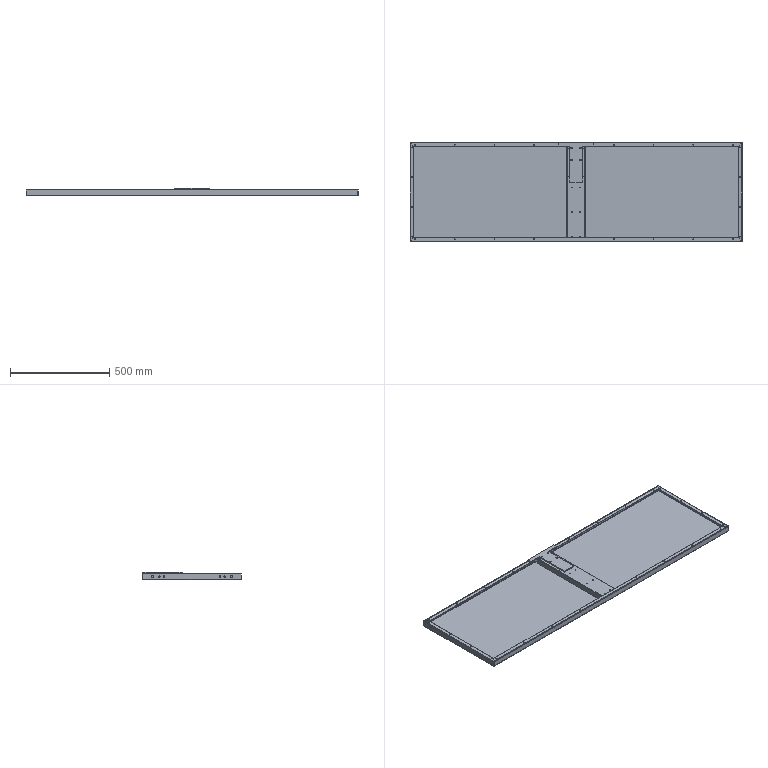Part | NX | features BREP 4 | 4 solids | 216 faces | box 1670 x 500 x 36 mm | volume 1279481 mm3 | cylinder 136 | plane 64 | spline 16 | commonest cylinder face diameters 4.5 x48 3.3 x20 6.8 x20 6.6 x16 1.473 x8 3.473 x8